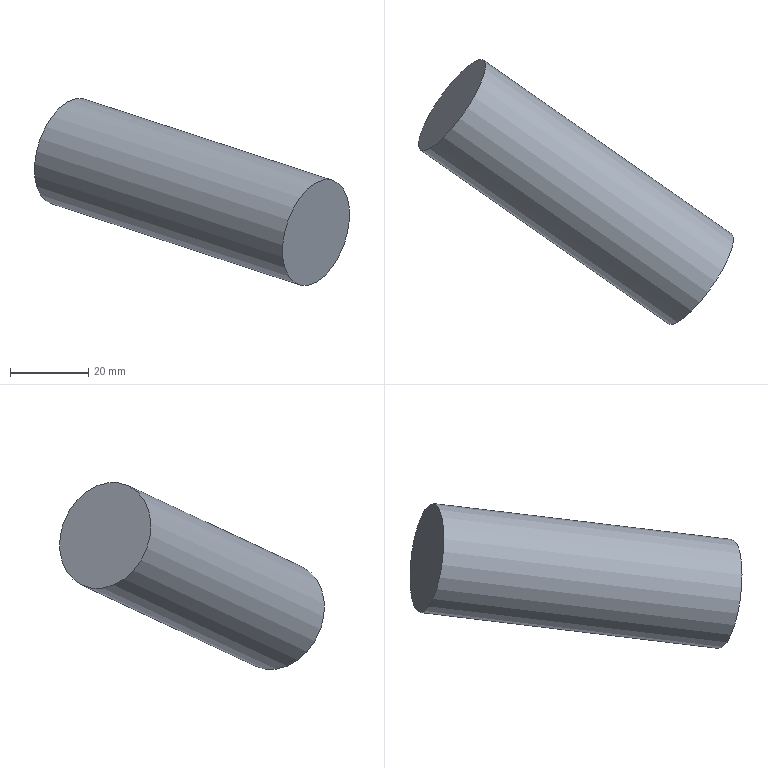Part | NX | features solid 2 | 1 solid | 3 faces | box 80.421 x 67.632 x 47.751 mm | volume 49260 mm3 | plane 2 | cylinder 1 | commonest cylinder face diameters 28 x1
STEP:
#1=CARTESIAN_POINT('',(-1037.451,617.782,-205.333));
#2=VERTEX_POINT('',#1);
#3=CARTESIAN_POINT('',(-1029.421,629.25,-205.333));
#4=DIRECTION('',(-0.7912,0.554,0.2588));
#5=DIRECTION('',(-0.5736,-0.8192,0.));
#6=AXIS2_PLACEMENT_3D('',#3,#4,#5);
#7=CIRCLE('',#6,14.);
#8=EDGE_CURVE('',#2,#2,#7,.T.);
#9=ORIENTED_EDGE('',*,*,#8,.F.);
#10=EDGE_LOOP('',(#9));
#11=FACE_BOUND('',#10,.T.);
#12=CARTESIAN_POINT('',(-974.152,573.46,-226.039));
#13=VERTEX_POINT('',#12);
#14=CARTESIAN_POINT('',(-966.122,584.928,-226.039));
#15=DIRECTION('',(-0.7912,0.554,0.2588));
#16=DIRECTION('',(-0.5736,-0.8192,0.));
#17=AXIS2_PLACEMENT_3D('',#14,#15,#16);
#18=CIRCLE('',#17,14.);
#19=EDGE_CURVE('',#13,#13,#18,.T.);
#20=ORIENTED_EDGE('',*,*,#19,.T.);
#21=EDGE_LOOP('',(#20));
#22=FACE_BOUND('',#21,.T.);
#23=CARTESIAN_POINT('',(-956.627,578.279,-229.144));
#24=DIRECTION('',(0.7912,-0.554,-0.2588));
#25=DIRECTION('',(0.5736,0.8192,0.));
#26=AXIS2_PLACEMENT_3D('',#23,#24,#25);
#27=CYLINDRICAL_SURFACE('',#26,14.);
#28=ADVANCED_FACE('',(#11,#22),#27,.T.);
#29=ORIENTED_EDGE('',*,*,#8,.T.);
#30=EDGE_LOOP('',(#29));
#31=FACE_BOUND('',#30,.T.);
#32=CARTESIAN_POINT('',(-1028.043,628.285,-199.055));
#33=DIRECTION('',(-0.7912,0.554,0.2588));
#34=DIRECTION('',(-0.5736,-0.8192,0.));
#35=AXIS2_PLACEMENT_3D('',#32,#33,#34);
#36=PLANE('',#35);
#37=ADVANCED_FACE('',(#31),#36,.T.);
#38=ORIENTED_EDGE('',*,*,#19,.F.);
#39=EDGE_LOOP('',(#38));
#40=FACE_BOUND('',#39,.T.);
#41=CARTESIAN_POINT('',(-964.744,583.963,-219.76));
#42=DIRECTION('',(-0.7912,0.554,0.2588));
#43=DIRECTION('',(-0.5736,-0.8192,0.));
#44=AXIS2_PLACEMENT_3D('',#41,#42,#43);
#45=PLANE('',#44);
#46=ADVANCED_FACE('',(#40),#45,.F.);
#47=CLOSED_SHELL('',(#28,#37,#46));
#48=MANIFOLD_SOLID_BREP('',#47);
#49=(LENGTH_UNIT()NAMED_UNIT(*)SI_UNIT(.MILLI.,.METRE.));
#50=UNCERTAINTY_MEASURE_WITH_UNIT(LENGTH_MEASURE(0.00001),#49,'','');
#51=(NAMED_UNIT(*)PLANE_ANGLE_UNIT()SI_UNIT($,.RADIAN.));
#52=(NAMED_UNIT(*)SI_UNIT($,.STERADIAN.)SOLID_ANGLE_UNIT());
#53=(GEOMETRIC_REPRESENTATION_CONTEXT(3)GLOBAL_UNCERTAINTY_ASSIGNED_CONTEXT((#50))GLOBAL_UNIT_ASSIGNED_CONTEXT((#49,#51,#52))REPRESENTATION_CONTEXT('',''));
#54=ADVANCED_BREP_SHAPE_REPRESENTATION('',(#48),#53);